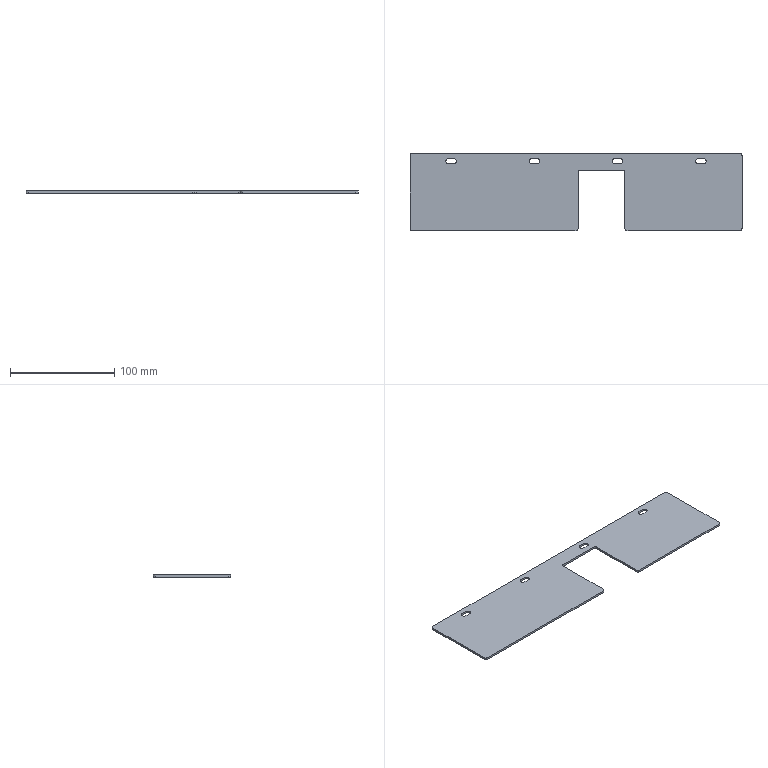Part | STEP file | 1 solid | 38 faces | box 319 x 74 x 2 mm | volume 41628 mm3 | cylinder 20 | plane 18 | commonest cylinder face diameters 5 x12 4 x8